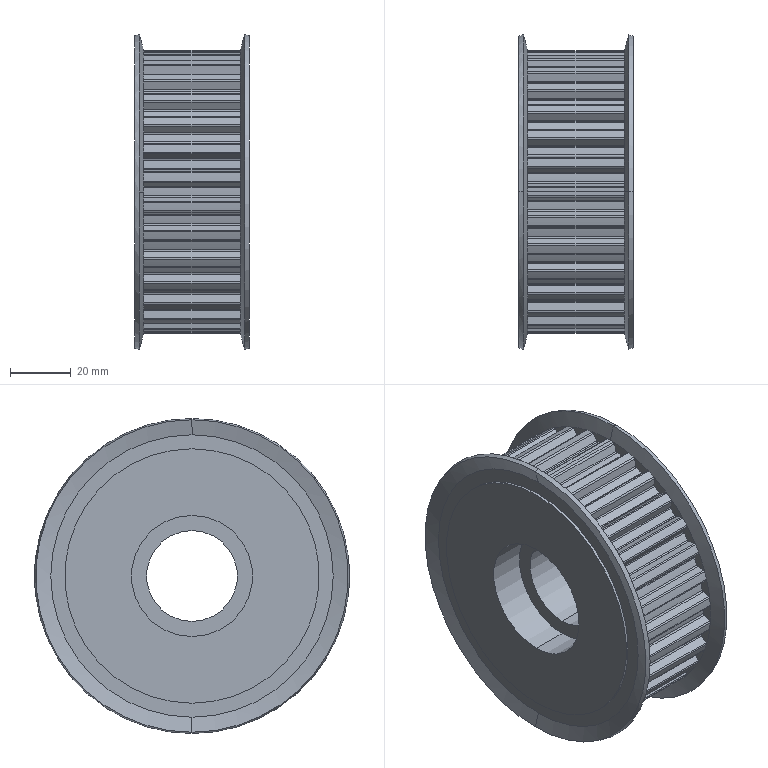Part | SolidWorks | features ICE 3, BaseBody 1 | 1 solid | 349 faces | box 37.864 x 104 x 104 mm | volume 203249 mm3 | cylinder 211 | plane 126 | cone 12 | commonest cylinder face diameters 1 x70 1.2 x70 93.65 x31 87.25 x30 40 x4 84 x4